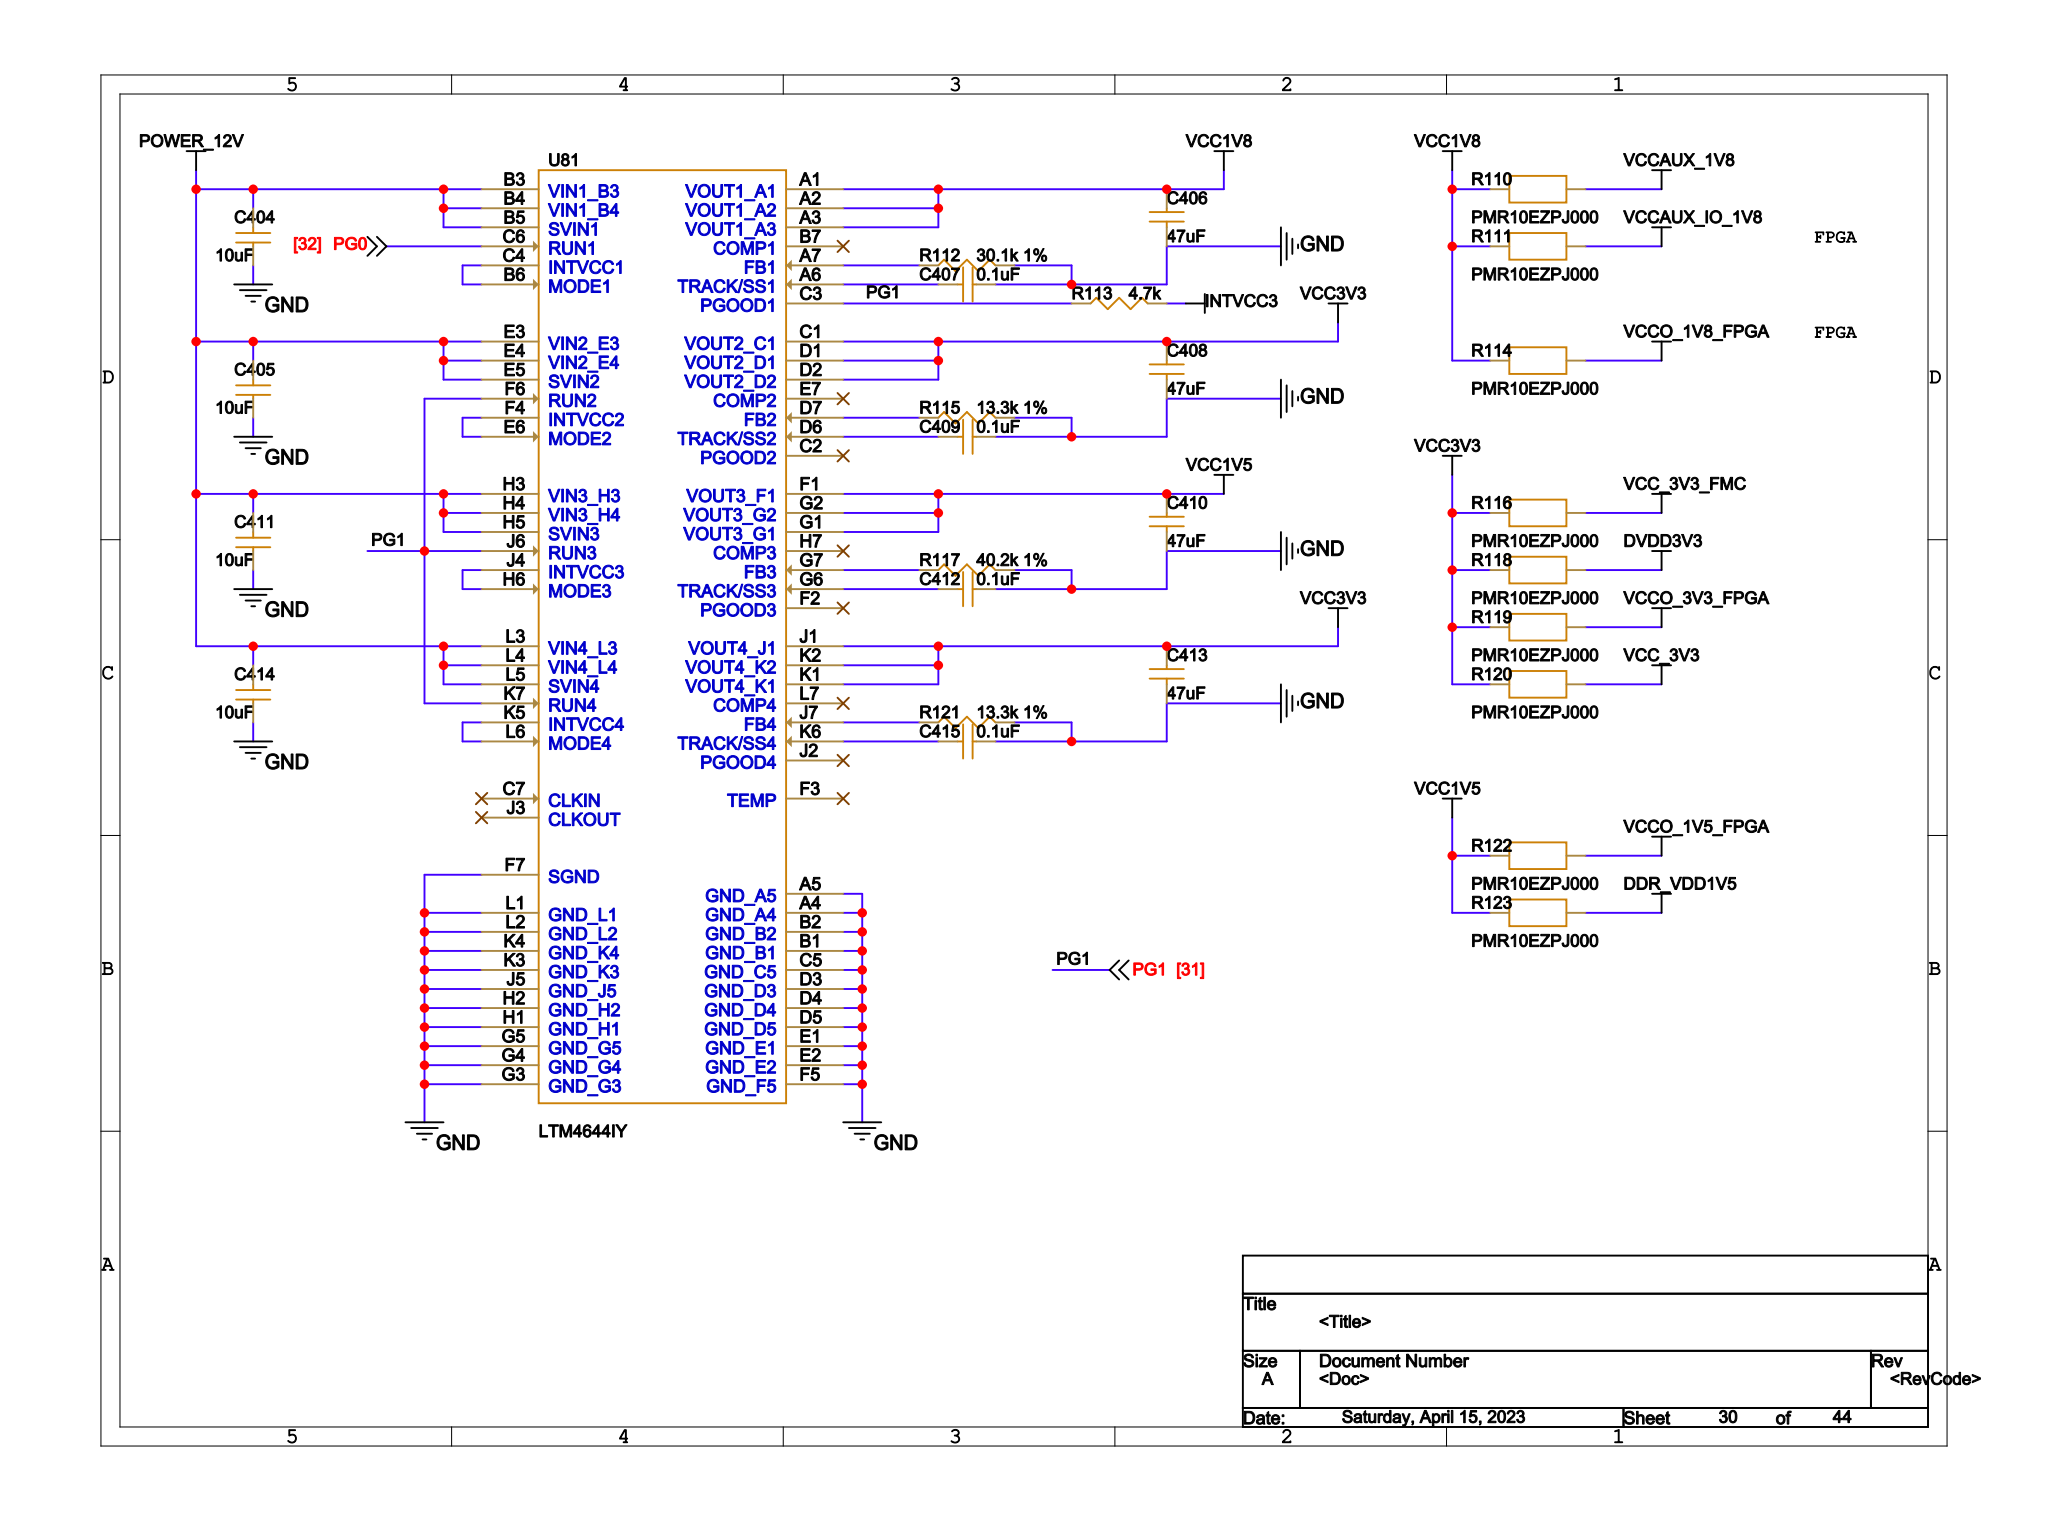Circuit board | Cadence Allegro | 1034 parts | 912 nets | one sheet of the schematic
Parts on this sheet (reference | value | footprint):
C404 | 10uF | C0402
C405 | 10uF | C0402
C406 | 47uF | C0402
C407 | 0.1uF | C0402
C408 | 47uF | C0402
C409 | 0.1uF | C0402
C410 | 47uF | C0402
C411 | 10uF | C0402
C412 | 0.1uF | C0402
C413 | 47uF | C0402
C414 | 10uF | C0402
C415 | 0.1uF | C0402
R110 | PMR10EZPJ000 | PMR0805
R111 | PMR10EZPJ000 | PMR0805
R112 | 30.1k 1% | R0402
R113 | 4.7k | R0402
R114 | PMR10EZPJ000 | PMR0805
R115 | 13.3k 1% | R0402
R116 | PMR10EZPJ000 | PMR0805
R117 | 40.2k 1% | R0402
R118 | PMR10EZPJ000 | PMR0805
R119 | PMR10EZPJ000 | PMR0805
R120 | PMR10EZPJ000 | PMR0805
R121 | 13.3k 1% | R0402
R122 | PMR10EZPJ000 | PMR0805
R123 | PMR10EZPJ000 | PMR0805
U81 | LTM4644IY | BGA77-1_27-15_0X9_0-H5_21
Nets of these parts (net: part-pin ...):
GND: C404-1 C405-1 C406-2 C407-1 C408-2 C409-1 C410-2 C411-1 C412-1 C413-2 C414-1 C415-1 R112-2 R115-2 R117-2 R121-2 U81-A4 U81-A5 U81-B1 U81-B2 U81-C5 U81-D3 U81-D4 U81-D5 U81-E1 U81-E2 U81-F5 U81-F7 U81-G3 U81-G4 U81-G5 U81-H1 U81-H2 U81-J5 U81-K3 U81-K4 U81-L1 U81-L2
VCC_3V3: R120-2
VCCO_3V3_FPGA: R119-2
VCCAUX_1V8: R110-2
VCCAUX_IO_1V8: R111-2
VCCO_1V5_FPGA: R122-2
VCCO_1V8_FPGA: R114-2
DVDD3V3: R118-2
DDR_VDD1V5: R123-2
N412962: C409-2 U81-D6
N406077: C412-2 U81-G6
N14327785: C415-2 U81-K6
N405379: C407-2 U81-A6
POWER_12V: C404-2 C405-2 C411-2 C414-2 U81-B3 U81-B4 U81-B5 U81-E3 U81-E4 U81-E5 U81-H3 U81-H4 U81-H5 U81-L3 U81-L4 U81-L5
VCC1V5: C410-1 R122-1 R123-1 U81-F1 U81-G1 U81-G2
VCC3V3: C408-1 C413-1 R116-1 R118-1 R119-1 R120-1 U81-C1 U81-D1 U81-D2 U81-J1 U81-K1 U81-K2
VCC1V8: C406-1 R110-1 R111-1 R114-1 U81-A1 U81-A2 U81-A3
INTVCC3: R113-2
VCC_3V3_FMC: R116-2
PG1: R113-1 U81-C3 U81-F6 U81-J6 U81-K7
N405375: R112-1 U81-A7
N412934: R115-1 U81-D7
N14327753: R121-1 U81-J7
N406057: R117-1 U81-G7
PG0: U81-C6